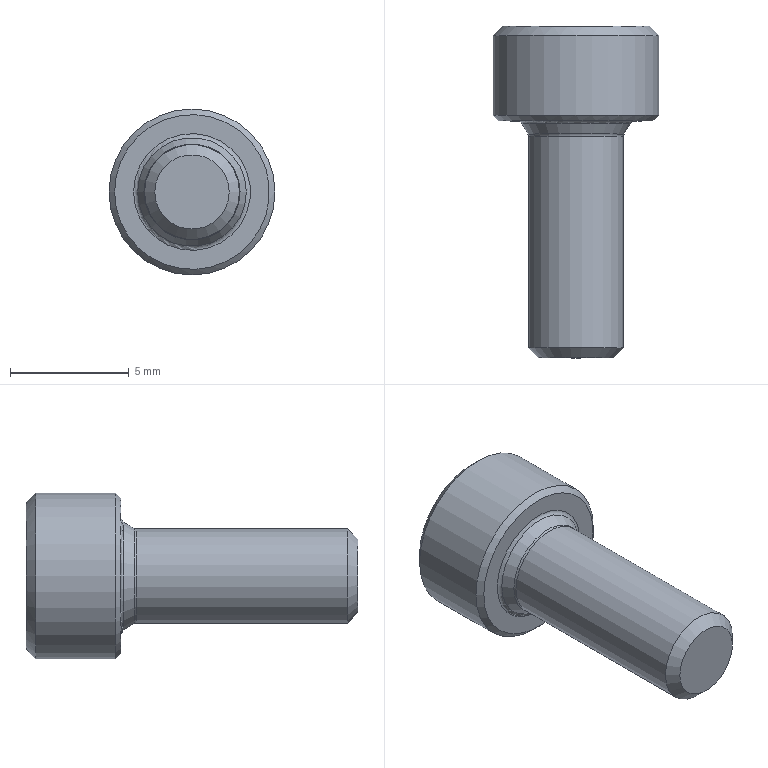Part | STEP file | 1 solid | 31 faces | box 7 x 14 x 7 mm | volume 255.725 mm3 | plane 15 | cone 11 | cylinder 3 | torus 2 | commonest cylinder face diameters 3 x1 4 x1 7 x1